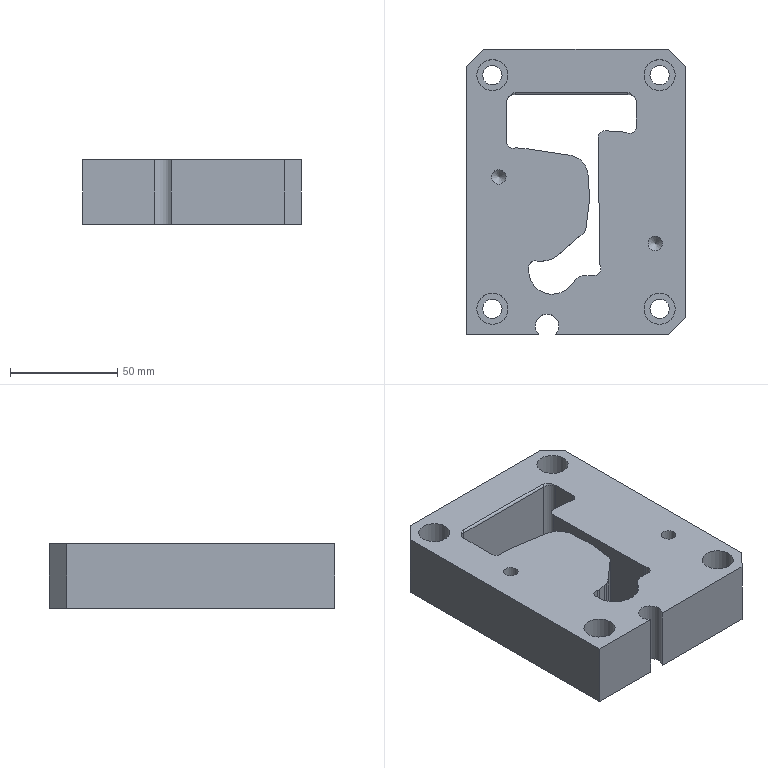Part | NX | features solid 2 | 1 solid | 62 faces | box 102 x 133 x 30 mm | volume 320641 mm3 | plane 32 | cylinder 26 | cone 2 | torus 2 | commonest cylinder face diameters 6 x9 9 x4 14.5 x4 6.8 x2 8 x2 2 x1